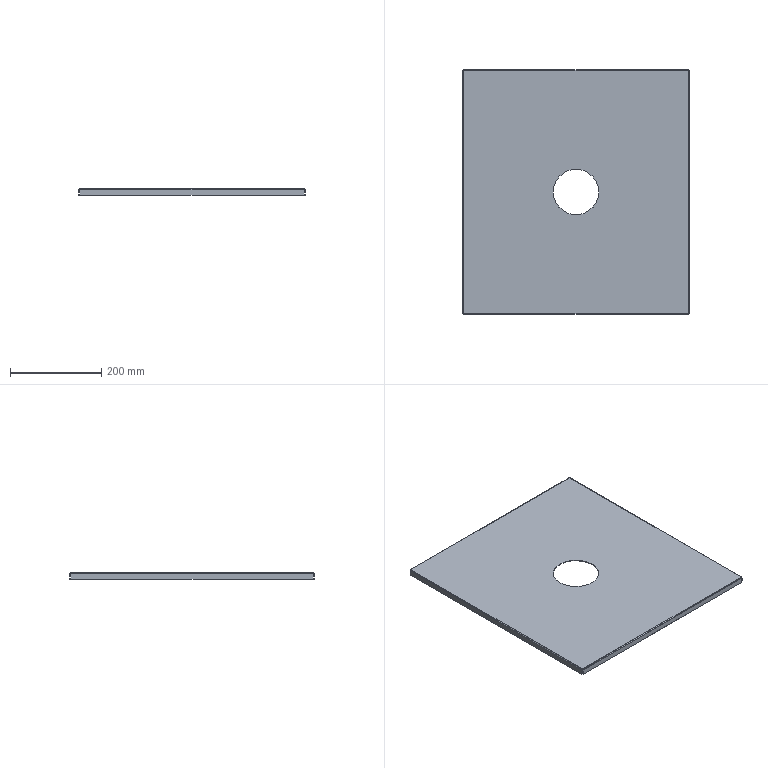Part | STEP file | Part 2^Frame unit | 1 solid | 40 faces | box 498 x 538 x 13.5 mm | volume 425403 mm3 | plane 22 | cylinder 10 | spline 8 | commonest cylinder face diameters 1 x4 4 x4 100 x2